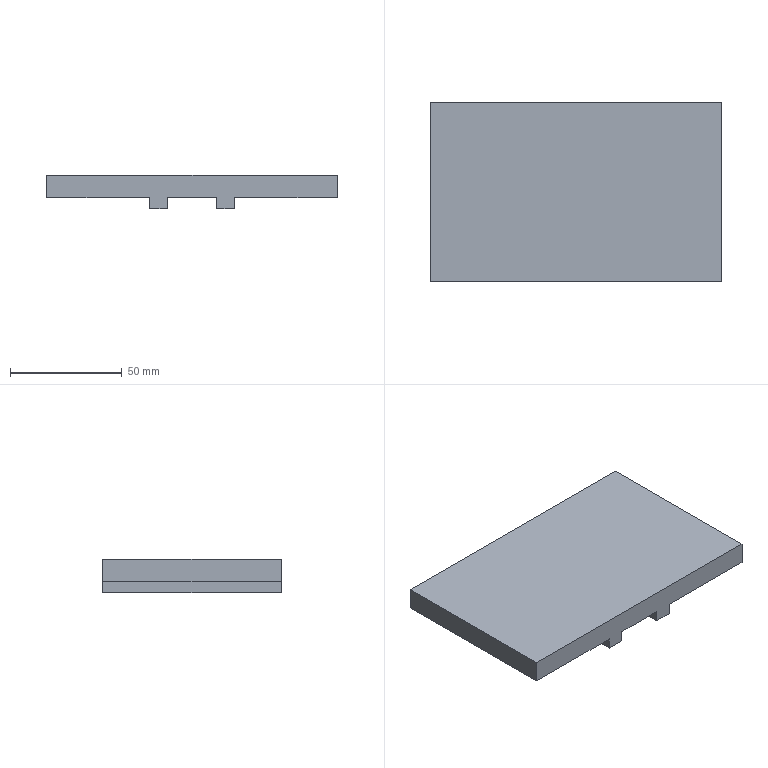Part | SolidWorks | features Extrusion 1, ICE 1 | 1 solid | 14 faces | box 130 x 80 x 15 mm | volume 110400 mm3 | plane 14
STEP:
#1=CARTESIAN_POINT('',(709.,79.,0.));
#2=VERTEX_POINT('',#1);
#3=CARTESIAN_POINT('',(731.,79.,0.));
#4=VERTEX_POINT('',#3);
#5=CARTESIAN_POINT('',(785.,79.,0.));
#6=DIRECTION('',(1.,0.,0.));
#7=VECTOR('',#6,1000.);
#8=LINE('',#5,#7);
#9=EDGE_CURVE('',#2,#4,#8,.T.);
#10=ORIENTED_EDGE('',*,*,#9,.F.);
#11=CARTESIAN_POINT('',(709.,159.,0.));
#12=VERTEX_POINT('',#11);
#13=CARTESIAN_POINT('',(709.,159.,0.));
#14=DIRECTION('',(0.,-1.,0.));
#15=VECTOR('',#14,1000.);
#16=LINE('',#13,#15);
#17=EDGE_CURVE('',#12,#2,#16,.T.);
#18=ORIENTED_EDGE('',*,*,#17,.F.);
#19=CARTESIAN_POINT('',(731.,159.,0.));
#20=VERTEX_POINT('',#19);
#21=CARTESIAN_POINT('',(785.,159.,0.));
#22=DIRECTION('',(-1.,0.,0.));
#23=VECTOR('',#22,1000.);
#24=LINE('',#21,#23);
#25=EDGE_CURVE('',#20,#12,#24,.T.);
#26=ORIENTED_EDGE('',*,*,#25,.F.);
#27=CARTESIAN_POINT('',(731.,79.,0.));
#28=DIRECTION('',(0.,1.,0.));
#29=VECTOR('',#28,1000.);
#30=LINE('',#27,#29);
#31=EDGE_CURVE('',#4,#20,#30,.T.);
#32=ORIENTED_EDGE('',*,*,#31,.F.);
#33=EDGE_LOOP('',(#10,#18,#26,#32));
#34=FACE_OUTER_BOUND('',#33,.T.);
#35=CARTESIAN_POINT('',(0.,0.,0.));
#36=DIRECTION('',(0.,0.,-1.));
#37=DIRECTION('',(-1.,0.,0.));
#38=AXIS2_PLACEMENT_3D('',#35,#36,#37);
#39=PLANE('',#38);
#40=ADVANCED_FACE('',(#34),#39,.T.);
#41=CARTESIAN_POINT('',(701.,159.,0.));
#42=VERTEX_POINT('',#41);
#43=CARTESIAN_POINT('',(655.,159.,0.));
#44=VERTEX_POINT('',#43);
#45=CARTESIAN_POINT('',(785.,159.,0.));
#46=DIRECTION('',(-1.,0.,0.));
#47=VECTOR('',#46,1000.);
#48=LINE('',#45,#47);
#49=EDGE_CURVE('',#42,#44,#48,.T.);
#50=ORIENTED_EDGE('',*,*,#49,.F.);
#51=CARTESIAN_POINT('',(701.,79.,0.));
#52=VERTEX_POINT('',#51);
#53=CARTESIAN_POINT('',(701.,79.,0.));
#54=DIRECTION('',(0.,1.,0.));
#55=VECTOR('',#54,1000.);
#56=LINE('',#53,#55);
#57=EDGE_CURVE('',#52,#42,#56,.T.);
#58=ORIENTED_EDGE('',*,*,#57,.F.);
#59=CARTESIAN_POINT('',(655.,79.,0.));
#60=VERTEX_POINT('',#59);
#61=CARTESIAN_POINT('',(785.,79.,0.));
#62=DIRECTION('',(1.,0.,0.));
#63=VECTOR('',#62,1000.);
#64=LINE('',#61,#63);
#65=EDGE_CURVE('',#60,#52,#64,.T.);
#66=ORIENTED_EDGE('',*,*,#65,.F.);
#67=CARTESIAN_POINT('',(655.,159.,0.));
#68=DIRECTION('',(0.,-1.,0.));
#69=VECTOR('',#68,1000.);
#70=LINE('',#67,#69);
#71=EDGE_CURVE('',#44,#60,#70,.T.);
#72=ORIENTED_EDGE('',*,*,#71,.F.);
#73=EDGE_LOOP('',(#50,#58,#66,#72));
#74=FACE_OUTER_BOUND('',#73,.T.);
#75=CARTESIAN_POINT('',(0.,0.,0.));
#76=DIRECTION('',(0.,0.,-1.));
#77=DIRECTION('',(-1.,0.,0.));
#78=AXIS2_PLACEMENT_3D('',#75,#76,#77);
#79=PLANE('',#78);
#80=ADVANCED_FACE('',(#74),#79,.T.);
#81=CARTESIAN_POINT('',(739.,159.,0.));
#82=VERTEX_POINT('',#81);
#83=CARTESIAN_POINT('',(739.,79.,0.));
#84=VERTEX_POINT('',#83);
#85=CARTESIAN_POINT('',(739.,159.,0.));
#86=DIRECTION('',(0.,-1.,0.));
#87=VECTOR('',#86,1000.);
#88=LINE('',#85,#87);
#89=EDGE_CURVE('',#82,#84,#88,.T.);
#90=ORIENTED_EDGE('',*,*,#89,.F.);
#91=CARTESIAN_POINT('',(785.,159.,0.));
#92=VERTEX_POINT('',#91);
#93=CARTESIAN_POINT('',(785.,159.,0.));
#94=DIRECTION('',(-1.,0.,0.));
#95=VECTOR('',#94,1000.);
#96=LINE('',#93,#95);
#97=EDGE_CURVE('',#92,#82,#96,.T.);
#98=ORIENTED_EDGE('',*,*,#97,.F.);
#99=CARTESIAN_POINT('',(785.,79.,0.));
#100=VERTEX_POINT('',#99);
#101=CARTESIAN_POINT('',(785.,159.,0.));
#102=DIRECTION('',(0.,1.,0.));
#103=VECTOR('',#102,1000.);
#104=LINE('',#101,#103);
#105=EDGE_CURVE('',#100,#92,#104,.T.);
#106=ORIENTED_EDGE('',*,*,#105,.F.);
#107=CARTESIAN_POINT('',(785.,79.,0.));
#108=DIRECTION('',(1.,0.,0.));
#109=VECTOR('',#108,1000.);
#110=LINE('',#107,#109);
#111=EDGE_CURVE('',#84,#100,#110,.T.);
#112=ORIENTED_EDGE('',*,*,#111,.F.);
#113=EDGE_LOOP('',(#90,#98,#106,#112));
#114=FACE_OUTER_BOUND('',#113,.T.);
#115=CARTESIAN_POINT('',(0.,0.,0.));
#116=DIRECTION('',(0.,0.,-1.));
#117=DIRECTION('',(-1.,0.,0.));
#118=AXIS2_PLACEMENT_3D('',#115,#116,#117);
#119=PLANE('',#118);
#120=ADVANCED_FACE('',(#114),#119,.T.);
#121=ORIENTED_EDGE('',*,*,#71,.T.);
#122=CARTESIAN_POINT('',(655.,79.,10.));
#123=VERTEX_POINT('',#122);
#124=CARTESIAN_POINT('',(655.,79.,10.));
#125=DIRECTION('',(0.,0.,-1.));
#126=VECTOR('',#125,1000.);
#127=LINE('',#124,#126);
#128=EDGE_CURVE('',#123,#60,#127,.T.);
#129=ORIENTED_EDGE('',*,*,#128,.F.);
#130=CARTESIAN_POINT('',(655.,159.,10.));
#131=VERTEX_POINT('',#130);
#132=CARTESIAN_POINT('',(655.,159.,10.));
#133=DIRECTION('',(0.,-1.,0.));
#134=VECTOR('',#133,1000.);
#135=LINE('',#132,#134);
#136=EDGE_CURVE('',#131,#123,#135,.T.);
#137=ORIENTED_EDGE('',*,*,#136,.F.);
#138=CARTESIAN_POINT('',(655.,159.,10.));
#139=DIRECTION('',(0.,0.,-1.));
#140=VECTOR('',#139,1000.);
#141=LINE('',#138,#140);
#142=EDGE_CURVE('',#131,#44,#141,.T.);
#143=ORIENTED_EDGE('',*,*,#142,.T.);
#144=EDGE_LOOP('',(#121,#129,#137,#143));
#145=FACE_OUTER_BOUND('',#144,.T.);
#146=CARTESIAN_POINT('',(655.,159.,10.));
#147=DIRECTION('',(1.,0.,0.));
#148=DIRECTION('',(0.,0.,-1.));
#149=AXIS2_PLACEMENT_3D('',#146,#147,#148);
#150=PLANE('',#149);
#151=ADVANCED_FACE('',(#145),#150,.F.);
#152=ORIENTED_EDGE('',*,*,#65,.T.);
#153=CARTESIAN_POINT('',(701.,79.,-5.));
#154=VERTEX_POINT('',#153);
#155=CARTESIAN_POINT('',(701.,79.,-85.399));
#156=DIRECTION('',(0.,0.,1.));
#157=VECTOR('',#156,1000.);
#158=LINE('',#155,#157);
#159=EDGE_CURVE('',#154,#52,#158,.T.);
#160=ORIENTED_EDGE('',*,*,#159,.F.);
#161=CARTESIAN_POINT('',(709.,79.,-5.));
#162=VERTEX_POINT('',#161);
#163=CARTESIAN_POINT('',(709.,79.,-5.));
#164=DIRECTION('',(-1.,0.,0.));
#165=VECTOR('',#164,1000.);
#166=LINE('',#163,#165);
#167=EDGE_CURVE('',#162,#154,#166,.T.);
#168=ORIENTED_EDGE('',*,*,#167,.F.);
#169=CARTESIAN_POINT('',(709.,79.,-85.399));
#170=DIRECTION('',(0.,0.,1.));
#171=VECTOR('',#170,1000.);
#172=LINE('',#169,#171);
#173=EDGE_CURVE('',#162,#2,#172,.T.);
#174=ORIENTED_EDGE('',*,*,#173,.T.);
#175=ORIENTED_EDGE('',*,*,#9,.T.);
#176=CARTESIAN_POINT('',(731.,79.,-5.));
#177=VERTEX_POINT('',#176);
#178=CARTESIAN_POINT('',(731.,79.,-85.399));
#179=DIRECTION('',(0.,0.,1.));
#180=VECTOR('',#179,1000.);
#181=LINE('',#178,#180);
#182=EDGE_CURVE('',#177,#4,#181,.T.);
#183=ORIENTED_EDGE('',*,*,#182,.F.);
#184=CARTESIAN_POINT('',(739.,79.,-5.));
#185=VERTEX_POINT('',#184);
#186=CARTESIAN_POINT('',(739.,79.,-5.));
#187=DIRECTION('',(-1.,0.,0.));
#188=VECTOR('',#187,1000.);
#189=LINE('',#186,#188);
#190=EDGE_CURVE('',#185,#177,#189,.T.);
#191=ORIENTED_EDGE('',*,*,#190,.F.);
#192=CARTESIAN_POINT('',(739.,79.,-85.399));
#193=DIRECTION('',(0.,0.,1.));
#194=VECTOR('',#193,1000.);
#195=LINE('',#192,#194);
#196=EDGE_CURVE('',#185,#84,#195,.T.);
#197=ORIENTED_EDGE('',*,*,#196,.T.);
#198=ORIENTED_EDGE('',*,*,#111,.T.);
#199=CARTESIAN_POINT('',(785.,79.,10.));
#200=VERTEX_POINT('',#199);
#201=CARTESIAN_POINT('',(785.,79.,10.));
#202=DIRECTION('',(0.,0.,-1.));
#203=VECTOR('',#202,1000.);
#204=LINE('',#201,#203);
#205=EDGE_CURVE('',#200,#100,#204,.T.);
#206=ORIENTED_EDGE('',*,*,#205,.F.);
#207=CARTESIAN_POINT('',(785.,79.,10.));
#208=DIRECTION('',(1.,0.,0.));
#209=VECTOR('',#208,1000.);
#210=LINE('',#207,#209);
#211=EDGE_CURVE('',#123,#200,#210,.T.);
#212=ORIENTED_EDGE('',*,*,#211,.F.);
#213=ORIENTED_EDGE('',*,*,#128,.T.);
#214=EDGE_LOOP('',(#152,#160,#168,#174,#175,#183,#191,#197,#198,#206,#212,#213));
#215=FACE_OUTER_BOUND('',#214,.T.);
#216=CARTESIAN_POINT('',(785.,79.,10.));
#217=DIRECTION('',(0.,1.,0.));
#218=DIRECTION('',(-1.,0.,0.));
#219=AXIS2_PLACEMENT_3D('',#216,#217,#218);
#220=PLANE('',#219);
#221=ADVANCED_FACE('',(#215),#220,.F.);
#222=ORIENTED_EDGE('',*,*,#105,.T.);
#223=CARTESIAN_POINT('',(785.,159.,10.));
#224=VERTEX_POINT('',#223);
#225=CARTESIAN_POINT('',(785.,159.,10.));
#226=DIRECTION('',(0.,0.,-1.));
#227=VECTOR('',#226,1000.);
#228=LINE('',#225,#227);
#229=EDGE_CURVE('',#224,#92,#228,.T.);
#230=ORIENTED_EDGE('',*,*,#229,.F.);
#231=CARTESIAN_POINT('',(785.,159.,10.));
#232=DIRECTION('',(0.,1.,0.));
#233=VECTOR('',#232,1000.);
#234=LINE('',#231,#233);
#235=EDGE_CURVE('',#200,#224,#234,.T.);
#236=ORIENTED_EDGE('',*,*,#235,.F.);
#237=ORIENTED_EDGE('',*,*,#205,.T.);
#238=EDGE_LOOP('',(#222,#230,#236,#237));
#239=FACE_OUTER_BOUND('',#238,.T.);
#240=CARTESIAN_POINT('',(785.,159.,10.));
#241=DIRECTION('',(-1.,0.,0.));
#242=DIRECTION('',(0.,-1.,0.));
#243=AXIS2_PLACEMENT_3D('',#240,#241,#242);
#244=PLANE('',#243);
#245=ADVANCED_FACE('',(#239),#244,.F.);
#246=ORIENTED_EDGE('',*,*,#97,.T.);
#247=CARTESIAN_POINT('',(739.,159.,-5.));
#248=VERTEX_POINT('',#247);
#249=CARTESIAN_POINT('',(739.,159.,-85.399));
#250=DIRECTION('',(0.,0.,1.));
#251=VECTOR('',#250,1000.);
#252=LINE('',#249,#251);
#253=EDGE_CURVE('',#248,#82,#252,.T.);
#254=ORIENTED_EDGE('',*,*,#253,.F.);
#255=CARTESIAN_POINT('',(731.,159.,-5.));
#256=VERTEX_POINT('',#255);
#257=CARTESIAN_POINT('',(739.,159.,-5.));
#258=DIRECTION('',(1.,0.,0.));
#259=VECTOR('',#258,1000.);
#260=LINE('',#257,#259);
#261=EDGE_CURVE('',#256,#248,#260,.T.);
#262=ORIENTED_EDGE('',*,*,#261,.F.);
#263=CARTESIAN_POINT('',(731.,159.,-85.399));
#264=DIRECTION('',(0.,0.,1.));
#265=VECTOR('',#264,1000.);
#266=LINE('',#263,#265);
#267=EDGE_CURVE('',#256,#20,#266,.T.);
#268=ORIENTED_EDGE('',*,*,#267,.T.);
#269=ORIENTED_EDGE('',*,*,#25,.T.);
#270=CARTESIAN_POINT('',(709.,159.,-5.));
#271=VERTEX_POINT('',#270);
#272=CARTESIAN_POINT('',(709.,159.,-85.399));
#273=DIRECTION('',(0.,0.,1.));
#274=VECTOR('',#273,1000.);
#275=LINE('',#272,#274);
#276=EDGE_CURVE('',#271,#12,#275,.T.);
#277=ORIENTED_EDGE('',*,*,#276,.F.);
#278=CARTESIAN_POINT('',(701.,159.,-5.));
#279=VERTEX_POINT('',#278);
#280=CARTESIAN_POINT('',(709.,159.,-5.));
#281=DIRECTION('',(1.,0.,0.));
#282=VECTOR('',#281,1000.);
#283=LINE('',#280,#282);
#284=EDGE_CURVE('',#279,#271,#283,.T.);
#285=ORIENTED_EDGE('',*,*,#284,.F.);
#286=CARTESIAN_POINT('',(701.,159.,-85.399));
#287=DIRECTION('',(0.,0.,1.));
#288=VECTOR('',#287,1000.);
#289=LINE('',#286,#288);
#290=EDGE_CURVE('',#279,#42,#289,.T.);
#291=ORIENTED_EDGE('',*,*,#290,.T.);
#292=ORIENTED_EDGE('',*,*,#49,.T.);
#293=ORIENTED_EDGE('',*,*,#142,.F.);
#294=CARTESIAN_POINT('',(785.,159.,10.));
#295=DIRECTION('',(-1.,0.,0.));
#296=VECTOR('',#295,1000.);
#297=LINE('',#294,#296);
#298=EDGE_CURVE('',#224,#131,#297,.T.);
#299=ORIENTED_EDGE('',*,*,#298,.F.);
#300=ORIENTED_EDGE('',*,*,#229,.T.);
#301=EDGE_LOOP('',(#246,#254,#262,#268,#269,#277,#285,#291,#292,#293,#299,#300));
#302=FACE_OUTER_BOUND('',#301,.T.);
#303=CARTESIAN_POINT('',(785.,159.,10.));
#304=DIRECTION('',(0.,-1.,0.));
#305=DIRECTION('',(1.,0.,0.));
#306=AXIS2_PLACEMENT_3D('',#303,#304,#305);
#307=PLANE('',#306);
#308=ADVANCED_FACE('',(#302),#307,.F.);
#309=ORIENTED_EDGE('',*,*,#136,.T.);
#310=ORIENTED_EDGE('',*,*,#211,.T.);
#311=ORIENTED_EDGE('',*,*,#235,.T.);
#312=ORIENTED_EDGE('',*,*,#298,.T.);
#313=EDGE_LOOP('',(#309,#310,#311,#312));
#314=FACE_OUTER_BOUND('',#313,.T.);
#315=CARTESIAN_POINT('',(0.,0.,10.));
#316=DIRECTION('',(0.,0.,-1.));
#317=DIRECTION('',(-1.,0.,0.));
#318=AXIS2_PLACEMENT_3D('',#315,#316,#317);
#319=PLANE('',#318);
#320=ADVANCED_FACE('',(#314),#319,.F.);
#321=CARTESIAN_POINT('',(739.,159.,-5.));
#322=DIRECTION('',(0.,-1.,0.));
#323=VECTOR('',#322,1000.);
#324=LINE('',#321,#323);
#325=EDGE_CURVE('',#248,#185,#324,.T.);
#326=ORIENTED_EDGE('',*,*,#325,.F.);
#327=ORIENTED_EDGE('',*,*,#253,.T.);
#328=ORIENTED_EDGE('',*,*,#89,.T.);
#329=ORIENTED_EDGE('',*,*,#196,.F.);
#330=EDGE_LOOP('',(#326,#327,#328,#329));
#331=FACE_OUTER_BOUND('',#330,.T.);
#332=CARTESIAN_POINT('',(739.,159.,-85.399));
#333=DIRECTION('',(-1.,0.,0.));
#334=DIRECTION('',(0.,0.,1.));
#335=AXIS2_PLACEMENT_3D('',#332,#333,#334);
#336=PLANE('',#335);
#337=ADVANCED_FACE('',(#331),#336,.F.);
#338=CARTESIAN_POINT('',(731.,79.,-5.));
#339=DIRECTION('',(0.,1.,0.));
#340=VECTOR('',#339,1000.);
#341=LINE('',#338,#340);
#342=EDGE_CURVE('',#177,#256,#341,.T.);
#343=ORIENTED_EDGE('',*,*,#342,.F.);
#344=ORIENTED_EDGE('',*,*,#182,.T.);
#345=ORIENTED_EDGE('',*,*,#31,.T.);
#346=ORIENTED_EDGE('',*,*,#267,.F.);
#347=EDGE_LOOP('',(#343,#344,#345,#346));
#348=FACE_OUTER_BOUND('',#347,.T.);
#349=CARTESIAN_POINT('',(731.,79.,-85.399));
#350=DIRECTION('',(1.,0.,0.));
#351=DIRECTION('',(0.,0.,-1.));
#352=AXIS2_PLACEMENT_3D('',#349,#350,#351);
#353=PLANE('',#352);
#354=ADVANCED_FACE('',(#348),#353,.F.);
#355=ORIENTED_EDGE('',*,*,#190,.T.);
#356=ORIENTED_EDGE('',*,*,#342,.T.);
#357=ORIENTED_EDGE('',*,*,#261,.T.);
#358=ORIENTED_EDGE('',*,*,#325,.T.);
#359=EDGE_LOOP('',(#355,#356,#357,#358));
#360=FACE_OUTER_BOUND('',#359,.T.);
#361=CARTESIAN_POINT('',(739.,-347.,-5.));
#362=DIRECTION('',(0.,0.,-1.));
#363=DIRECTION('',(0.,1.,0.));
#364=AXIS2_PLACEMENT_3D('',#361,#362,#363);
#365=PLANE('',#364);
#366=ADVANCED_FACE('',(#360),#365,.T.);
#367=CARTESIAN_POINT('',(709.,159.,-5.));
#368=DIRECTION('',(0.,-1.,0.));
#369=VECTOR('',#368,1000.);
#370=LINE('',#367,#369);
#371=EDGE_CURVE('',#271,#162,#370,.T.);
#372=ORIENTED_EDGE('',*,*,#371,.F.);
#373=ORIENTED_EDGE('',*,*,#276,.T.);
#374=ORIENTED_EDGE('',*,*,#17,.T.);
#375=ORIENTED_EDGE('',*,*,#173,.F.);
#376=EDGE_LOOP('',(#372,#373,#374,#375));
#377=FACE_OUTER_BOUND('',#376,.T.);
#378=CARTESIAN_POINT('',(709.,159.,-85.399));
#379=DIRECTION('',(-1.,0.,0.));
#380=DIRECTION('',(0.,0.,1.));
#381=AXIS2_PLACEMENT_3D('',#378,#379,#380);
#382=PLANE('',#381);
#383=ADVANCED_FACE('',(#377),#382,.F.);
#384=CARTESIAN_POINT('',(701.,79.,-5.));
#385=DIRECTION('',(0.,1.,0.));
#386=VECTOR('',#385,1000.);
#387=LINE('',#384,#386);
#388=EDGE_CURVE('',#154,#279,#387,.T.);
#389=ORIENTED_EDGE('',*,*,#388,.F.);
#390=ORIENTED_EDGE('',*,*,#159,.T.);
#391=ORIENTED_EDGE('',*,*,#57,.T.);
#392=ORIENTED_EDGE('',*,*,#290,.F.);
#393=EDGE_LOOP('',(#389,#390,#391,#392));
#394=FACE_OUTER_BOUND('',#393,.T.);
#395=CARTESIAN_POINT('',(701.,79.,-85.399));
#396=DIRECTION('',(1.,0.,0.));
#397=DIRECTION('',(0.,0.,-1.));
#398=AXIS2_PLACEMENT_3D('',#395,#396,#397);
#399=PLANE('',#398);
#400=ADVANCED_FACE('',(#394),#399,.F.);
#401=ORIENTED_EDGE('',*,*,#284,.T.);
#402=ORIENTED_EDGE('',*,*,#371,.T.);
#403=ORIENTED_EDGE('',*,*,#167,.T.);
#404=ORIENTED_EDGE('',*,*,#388,.T.);
#405=EDGE_LOOP('',(#401,#402,#403,#404));
#406=FACE_OUTER_BOUND('',#405,.T.);
#407=CARTESIAN_POINT('',(739.,-347.,-5.));
#408=DIRECTION('',(0.,0.,-1.));
#409=DIRECTION('',(0.,1.,0.));
#410=AXIS2_PLACEMENT_3D('',#407,#408,#409);
#411=PLANE('',#410);
#412=ADVANCED_FACE('',(#406),#411,.T.);
#413=CLOSED_SHELL('',(#40,#80,#120,#151,#221,#245,#308,#320,#337,#354,#366,#383,#400,#412));
#414=MANIFOLD_SOLID_BREP('',#413);
#415=CARTESIAN_POINT('',(0.,0.,0.));
#416=DIRECTION('',(0.,0.,1.));
#417=DIRECTION('',(1.,0.,0.));
#418=AXIS2_PLACEMENT_3D('',#415,#416,#417);
#419=(LENGTH_UNIT()NAMED_UNIT(*)SI_UNIT(.MILLI.,.METRE.));
#420=UNCERTAINTY_MEASURE_WITH_UNIT(LENGTH_MEASURE(0.00001),#419,'','');
#421=(NAMED_UNIT(*)PLANE_ANGLE_UNIT()SI_UNIT($,.RADIAN.));
#422=(NAMED_UNIT(*)SI_UNIT($,.STERADIAN.)SOLID_ANGLE_UNIT());
#423=(GEOMETRIC_REPRESENTATION_CONTEXT(3)GLOBAL_UNCERTAINTY_ASSIGNED_CONTEXT((#420))GLOBAL_UNIT_ASSIGNED_CONTEXT((#419,#421,#422))REPRESENTATION_CONTEXT('',''));
#424=ADVANCED_BREP_SHAPE_REPRESENTATION('',(#414,#418),#423);